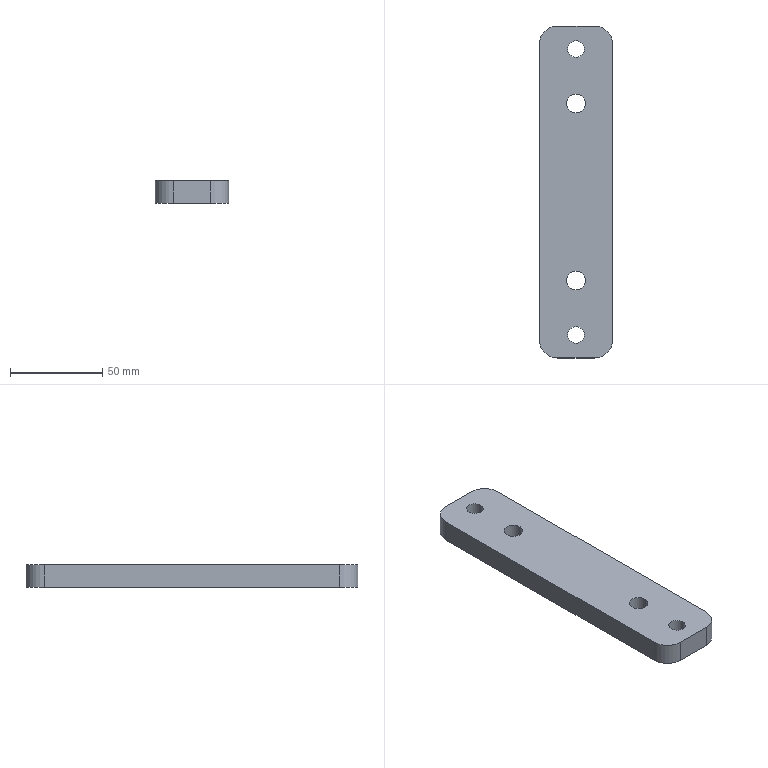Part | STEP file | Base plate 2_Default<Machined> | 1 solid | 18 faces | box 40 x 180 x 12 mm | volume 81882 mm3 | cylinder 12 | plane 6 | commonest cylinder face diameters 9 x4 10.2 x4 20 x4
STEP:
#1=CARTESIAN_POINT('',(-4.5,77.5,0.));
#2=VERTEX_POINT('',#1);
#3=CARTESIAN_POINT('',(4.5,77.5,0.));
#4=VERTEX_POINT('',#3);
#5=CARTESIAN_POINT('',(0.,77.5,0.));
#6=DIRECTION('',(0.,0.,1.));
#7=DIRECTION('',(1.,0.,0.));
#8=AXIS2_PLACEMENT_3D('',#5,#6,#7);
#9=CIRCLE('',#8,4.5);
#10=EDGE_CURVE('',#2,#4,#9,.T.);
#11=ORIENTED_EDGE('',*,*,#10,.F.);
#12=CARTESIAN_POINT('',(-4.5,77.5,12.));
#13=VERTEX_POINT('',#12);
#14=CARTESIAN_POINT('',(-4.5,77.5,12.));
#15=DIRECTION('',(0.,0.,1.));
#16=VECTOR('',#15,1000.);
#17=LINE('',#14,#16);
#18=EDGE_CURVE('',#2,#13,#17,.T.);
#19=ORIENTED_EDGE('',*,*,#18,.T.);
#20=CARTESIAN_POINT('',(4.5,77.5,12.));
#21=VERTEX_POINT('',#20);
#22=CARTESIAN_POINT('',(0.,77.5,12.));
#23=DIRECTION('',(0.,0.,1.));
#24=DIRECTION('',(1.,0.,0.));
#25=AXIS2_PLACEMENT_3D('',#22,#23,#24);
#26=CIRCLE('',#25,4.5);
#27=EDGE_CURVE('',#13,#21,#26,.T.);
#28=ORIENTED_EDGE('',*,*,#27,.T.);
#29=CARTESIAN_POINT('',(4.5,77.5,12.));
#30=DIRECTION('',(0.,0.,1.));
#31=VECTOR('',#30,1000.);
#32=LINE('',#29,#31);
#33=EDGE_CURVE('',#4,#21,#32,.T.);
#34=ORIENTED_EDGE('',*,*,#33,.F.);
#35=EDGE_LOOP('',(#11,#19,#28,#34));
#36=FACE_OUTER_BOUND('',#35,.T.);
#37=CARTESIAN_POINT('',(0.,77.5,12.));
#38=DIRECTION('',(0.,0.,1.));
#39=DIRECTION('',(1.,0.,0.));
#40=AXIS2_PLACEMENT_3D('',#37,#38,#39);
#41=CYLINDRICAL_SURFACE('',#40,4.5);
#42=ADVANCED_FACE('',(#36),#41,.F.);
#43=CARTESIAN_POINT('',(-4.5,-77.5,0.));
#44=VERTEX_POINT('',#43);
#45=CARTESIAN_POINT('',(4.5,-77.5,0.));
#46=VERTEX_POINT('',#45);
#47=CARTESIAN_POINT('',(0.,-77.5,0.));
#48=DIRECTION('',(0.,0.,1.));
#49=DIRECTION('',(1.,0.,0.));
#50=AXIS2_PLACEMENT_3D('',#47,#48,#49);
#51=CIRCLE('',#50,4.5);
#52=EDGE_CURVE('',#44,#46,#51,.T.);
#53=ORIENTED_EDGE('',*,*,#52,.F.);
#54=CARTESIAN_POINT('',(-4.5,-77.5,12.));
#55=VERTEX_POINT('',#54);
#56=CARTESIAN_POINT('',(-4.5,-77.5,12.));
#57=DIRECTION('',(0.,0.,1.));
#58=VECTOR('',#57,1000.);
#59=LINE('',#56,#58);
#60=EDGE_CURVE('',#44,#55,#59,.T.);
#61=ORIENTED_EDGE('',*,*,#60,.T.);
#62=CARTESIAN_POINT('',(4.5,-77.5,12.));
#63=VERTEX_POINT('',#62);
#64=CARTESIAN_POINT('',(0.,-77.5,12.));
#65=DIRECTION('',(0.,0.,1.));
#66=DIRECTION('',(1.,0.,0.));
#67=AXIS2_PLACEMENT_3D('',#64,#65,#66);
#68=CIRCLE('',#67,4.5);
#69=EDGE_CURVE('',#55,#63,#68,.T.);
#70=ORIENTED_EDGE('',*,*,#69,.T.);
#71=CARTESIAN_POINT('',(4.5,-77.5,12.));
#72=DIRECTION('',(0.,0.,1.));
#73=VECTOR('',#72,1000.);
#74=LINE('',#71,#73);
#75=EDGE_CURVE('',#46,#63,#74,.T.);
#76=ORIENTED_EDGE('',*,*,#75,.F.);
#77=EDGE_LOOP('',(#53,#61,#70,#76));
#78=FACE_OUTER_BOUND('',#77,.T.);
#79=CARTESIAN_POINT('',(0.,-77.5,12.));
#80=DIRECTION('',(0.,0.,1.));
#81=DIRECTION('',(1.,0.,0.));
#82=AXIS2_PLACEMENT_3D('',#79,#80,#81);
#83=CYLINDRICAL_SURFACE('',#82,4.5);
#84=ADVANCED_FACE('',(#78),#83,.F.);
#85=CARTESIAN_POINT('',(-5.1,48.,0.));
#86=VERTEX_POINT('',#85);
#87=CARTESIAN_POINT('',(5.1,48.,0.));
#88=VERTEX_POINT('',#87);
#89=CARTESIAN_POINT('',(0.,48.,0.));
#90=DIRECTION('',(0.,0.,1.));
#91=DIRECTION('',(1.,0.,0.));
#92=AXIS2_PLACEMENT_3D('',#89,#90,#91);
#93=CIRCLE('',#92,5.1);
#94=EDGE_CURVE('',#86,#88,#93,.T.);
#95=ORIENTED_EDGE('',*,*,#94,.F.);
#96=CARTESIAN_POINT('',(-5.1,48.,12.));
#97=VERTEX_POINT('',#96);
#98=CARTESIAN_POINT('',(-5.1,48.,12.));
#99=DIRECTION('',(0.,0.,1.));
#100=VECTOR('',#99,1000.);
#101=LINE('',#98,#100);
#102=EDGE_CURVE('',#86,#97,#101,.T.);
#103=ORIENTED_EDGE('',*,*,#102,.T.);
#104=CARTESIAN_POINT('',(5.1,48.,12.));
#105=VERTEX_POINT('',#104);
#106=CARTESIAN_POINT('',(0.,48.,12.));
#107=DIRECTION('',(0.,0.,1.));
#108=DIRECTION('',(1.,0.,0.));
#109=AXIS2_PLACEMENT_3D('',#106,#107,#108);
#110=CIRCLE('',#109,5.1);
#111=EDGE_CURVE('',#97,#105,#110,.T.);
#112=ORIENTED_EDGE('',*,*,#111,.T.);
#113=CARTESIAN_POINT('',(5.1,48.,12.));
#114=DIRECTION('',(0.,0.,1.));
#115=VECTOR('',#114,1000.);
#116=LINE('',#113,#115);
#117=EDGE_CURVE('',#88,#105,#116,.T.);
#118=ORIENTED_EDGE('',*,*,#117,.F.);
#119=EDGE_LOOP('',(#95,#103,#112,#118));
#120=FACE_OUTER_BOUND('',#119,.T.);
#121=CARTESIAN_POINT('',(0.,48.,12.));
#122=DIRECTION('',(0.,0.,1.));
#123=DIRECTION('',(1.,0.,0.));
#124=AXIS2_PLACEMENT_3D('',#121,#122,#123);
#125=CYLINDRICAL_SURFACE('',#124,5.1);
#126=ADVANCED_FACE('',(#120),#125,.F.);
#127=CARTESIAN_POINT('',(-5.1,-48.,0.));
#128=VERTEX_POINT('',#127);
#129=CARTESIAN_POINT('',(5.1,-48.,0.));
#130=VERTEX_POINT('',#129);
#131=CARTESIAN_POINT('',(0.,-48.,0.));
#132=DIRECTION('',(0.,0.,1.));
#133=DIRECTION('',(1.,0.,0.));
#134=AXIS2_PLACEMENT_3D('',#131,#132,#133);
#135=CIRCLE('',#134,5.1);
#136=EDGE_CURVE('',#128,#130,#135,.T.);
#137=ORIENTED_EDGE('',*,*,#136,.F.);
#138=CARTESIAN_POINT('',(-5.1,-48.,12.));
#139=VERTEX_POINT('',#138);
#140=CARTESIAN_POINT('',(-5.1,-48.,12.));
#141=DIRECTION('',(0.,0.,1.));
#142=VECTOR('',#141,1000.);
#143=LINE('',#140,#142);
#144=EDGE_CURVE('',#128,#139,#143,.T.);
#145=ORIENTED_EDGE('',*,*,#144,.T.);
#146=CARTESIAN_POINT('',(5.1,-48.,12.));
#147=VERTEX_POINT('',#146);
#148=CARTESIAN_POINT('',(0.,-48.,12.));
#149=DIRECTION('',(0.,0.,1.));
#150=DIRECTION('',(1.,0.,0.));
#151=AXIS2_PLACEMENT_3D('',#148,#149,#150);
#152=CIRCLE('',#151,5.1);
#153=EDGE_CURVE('',#139,#147,#152,.T.);
#154=ORIENTED_EDGE('',*,*,#153,.T.);
#155=CARTESIAN_POINT('',(5.1,-48.,12.));
#156=DIRECTION('',(0.,0.,1.));
#157=VECTOR('',#156,1000.);
#158=LINE('',#155,#157);
#159=EDGE_CURVE('',#130,#147,#158,.T.);
#160=ORIENTED_EDGE('',*,*,#159,.F.);
#161=EDGE_LOOP('',(#137,#145,#154,#160));
#162=FACE_OUTER_BOUND('',#161,.T.);
#163=CARTESIAN_POINT('',(0.,-48.,12.));
#164=DIRECTION('',(0.,0.,1.));
#165=DIRECTION('',(1.,0.,0.));
#166=AXIS2_PLACEMENT_3D('',#163,#164,#165);
#167=CYLINDRICAL_SURFACE('',#166,5.1);
#168=ADVANCED_FACE('',(#162),#167,.F.);
#169=CARTESIAN_POINT('',(20.,-80.,12.));
#170=VERTEX_POINT('',#169);
#171=CARTESIAN_POINT('',(20.,80.,12.));
#172=VERTEX_POINT('',#171);
#173=CARTESIAN_POINT('',(20.,90.,12.));
#174=DIRECTION('',(0.,1.,0.));
#175=VECTOR('',#174,1000.);
#176=LINE('',#173,#175);
#177=EDGE_CURVE('',#170,#172,#176,.T.);
#178=ORIENTED_EDGE('',*,*,#177,.F.);
#179=CARTESIAN_POINT('',(20.,-80.,0.));
#180=VERTEX_POINT('',#179);
#181=CARTESIAN_POINT('',(20.,-80.,12.));
#182=DIRECTION('',(0.,0.,-1.));
#183=VECTOR('',#182,1000.);
#184=LINE('',#181,#183);
#185=EDGE_CURVE('',#170,#180,#184,.T.);
#186=ORIENTED_EDGE('',*,*,#185,.T.);
#187=CARTESIAN_POINT('',(20.,80.,0.));
#188=VERTEX_POINT('',#187);
#189=CARTESIAN_POINT('',(20.,90.,0.));
#190=DIRECTION('',(0.,1.,0.));
#191=VECTOR('',#190,1000.);
#192=LINE('',#189,#191);
#193=EDGE_CURVE('',#180,#188,#192,.T.);
#194=ORIENTED_EDGE('',*,*,#193,.T.);
#195=CARTESIAN_POINT('',(20.,80.,12.));
#196=DIRECTION('',(0.,0.,1.));
#197=VECTOR('',#196,1000.);
#198=LINE('',#195,#197);
#199=EDGE_CURVE('',#188,#172,#198,.T.);
#200=ORIENTED_EDGE('',*,*,#199,.T.);
#201=EDGE_LOOP('',(#178,#186,#194,#200));
#202=FACE_OUTER_BOUND('',#201,.T.);
#203=CARTESIAN_POINT('',(20.,90.,12.));
#204=DIRECTION('',(-1.,0.,0.));
#205=DIRECTION('',(0.,-1.,0.));
#206=AXIS2_PLACEMENT_3D('',#203,#204,#205);
#207=PLANE('',#206);
#208=ADVANCED_FACE('',(#202),#207,.F.);
#209=CARTESIAN_POINT('',(10.,90.,12.));
#210=VERTEX_POINT('',#209);
#211=CARTESIAN_POINT('',(-10.,90.,12.));
#212=VERTEX_POINT('',#211);
#213=CARTESIAN_POINT('',(-20.,90.,12.));
#214=DIRECTION('',(-1.,0.,0.));
#215=VECTOR('',#214,1000.);
#216=LINE('',#213,#215);
#217=EDGE_CURVE('',#210,#212,#216,.T.);
#218=ORIENTED_EDGE('',*,*,#217,.F.);
#219=CARTESIAN_POINT('',(10.,90.,0.));
#220=VERTEX_POINT('',#219);
#221=CARTESIAN_POINT('',(10.,90.,12.));
#222=DIRECTION('',(0.,0.,-1.));
#223=VECTOR('',#222,1000.);
#224=LINE('',#221,#223);
#225=EDGE_CURVE('',#210,#220,#224,.T.);
#226=ORIENTED_EDGE('',*,*,#225,.T.);
#227=CARTESIAN_POINT('',(-10.,90.,0.));
#228=VERTEX_POINT('',#227);
#229=CARTESIAN_POINT('',(-20.,90.,0.));
#230=DIRECTION('',(-1.,0.,0.));
#231=VECTOR('',#230,1000.);
#232=LINE('',#229,#231);
#233=EDGE_CURVE('',#220,#228,#232,.T.);
#234=ORIENTED_EDGE('',*,*,#233,.T.);
#235=CARTESIAN_POINT('',(-10.,90.,12.));
#236=DIRECTION('',(0.,0.,1.));
#237=VECTOR('',#236,1000.);
#238=LINE('',#235,#237);
#239=EDGE_CURVE('',#228,#212,#238,.T.);
#240=ORIENTED_EDGE('',*,*,#239,.T.);
#241=EDGE_LOOP('',(#218,#226,#234,#240));
#242=FACE_OUTER_BOUND('',#241,.T.);
#243=CARTESIAN_POINT('',(-20.,90.,12.));
#244=DIRECTION('',(0.,-1.,0.));
#245=DIRECTION('',(0.,0.,-1.));
#246=AXIS2_PLACEMENT_3D('',#243,#244,#245);
#247=PLANE('',#246);
#248=ADVANCED_FACE('',(#242),#247,.F.);
#249=CARTESIAN_POINT('',(-20.,80.,0.));
#250=VERTEX_POINT('',#249);
#251=CARTESIAN_POINT('',(-20.,-80.,0.));
#252=VERTEX_POINT('',#251);
#253=CARTESIAN_POINT('',(-20.,90.,0.));
#254=DIRECTION('',(0.,-1.,0.));
#255=VECTOR('',#254,1000.);
#256=LINE('',#253,#255);
#257=EDGE_CURVE('',#250,#252,#256,.T.);
#258=ORIENTED_EDGE('',*,*,#257,.T.);
#259=CARTESIAN_POINT('',(-20.,-80.,12.));
#260=VERTEX_POINT('',#259);
#261=CARTESIAN_POINT('',(-20.,-80.,12.));
#262=DIRECTION('',(0.,0.,1.));
#263=VECTOR('',#262,1000.);
#264=LINE('',#261,#263);
#265=EDGE_CURVE('',#252,#260,#264,.T.);
#266=ORIENTED_EDGE('',*,*,#265,.T.);
#267=CARTESIAN_POINT('',(-20.,80.,12.));
#268=VERTEX_POINT('',#267);
#269=CARTESIAN_POINT('',(-20.,90.,12.));
#270=DIRECTION('',(0.,-1.,0.));
#271=VECTOR('',#270,1000.);
#272=LINE('',#269,#271);
#273=EDGE_CURVE('',#268,#260,#272,.T.);
#274=ORIENTED_EDGE('',*,*,#273,.F.);
#275=CARTESIAN_POINT('',(-20.,80.,12.));
#276=DIRECTION('',(0.,0.,-1.));
#277=VECTOR('',#276,1000.);
#278=LINE('',#275,#277);
#279=EDGE_CURVE('',#268,#250,#278,.T.);
#280=ORIENTED_EDGE('',*,*,#279,.T.);
#281=EDGE_LOOP('',(#258,#266,#274,#280));
#282=FACE_OUTER_BOUND('',#281,.T.);
#283=CARTESIAN_POINT('',(-20.,90.,12.));
#284=DIRECTION('',(1.,0.,0.));
#285=DIRECTION('',(0.,1.,0.));
#286=AXIS2_PLACEMENT_3D('',#283,#284,#285);
#287=PLANE('',#286);
#288=ADVANCED_FACE('',(#282),#287,.F.);
#289=CARTESIAN_POINT('',(-10.,-90.,0.));
#290=VERTEX_POINT('',#289);
#291=CARTESIAN_POINT('',(10.,-90.,0.));
#292=VERTEX_POINT('',#291);
#293=CARTESIAN_POINT('',(-20.,-90.,0.));
#294=DIRECTION('',(1.,0.,0.));
#295=VECTOR('',#294,1000.);
#296=LINE('',#293,#295);
#297=EDGE_CURVE('',#290,#292,#296,.T.);
#298=ORIENTED_EDGE('',*,*,#297,.T.);
#299=CARTESIAN_POINT('',(10.,-90.,12.));
#300=VERTEX_POINT('',#299);
#301=CARTESIAN_POINT('',(10.,-90.,12.));
#302=DIRECTION('',(0.,0.,1.));
#303=VECTOR('',#302,1000.);
#304=LINE('',#301,#303);
#305=EDGE_CURVE('',#292,#300,#304,.T.);
#306=ORIENTED_EDGE('',*,*,#305,.T.);
#307=CARTESIAN_POINT('',(-10.,-90.,12.));
#308=VERTEX_POINT('',#307);
#309=CARTESIAN_POINT('',(-20.,-90.,12.));
#310=DIRECTION('',(1.,0.,0.));
#311=VECTOR('',#310,1000.);
#312=LINE('',#309,#311);
#313=EDGE_CURVE('',#308,#300,#312,.T.);
#314=ORIENTED_EDGE('',*,*,#313,.F.);
#315=CARTESIAN_POINT('',(-10.,-90.,12.));
#316=DIRECTION('',(0.,0.,-1.));
#317=VECTOR('',#316,1000.);
#318=LINE('',#315,#317);
#319=EDGE_CURVE('',#308,#290,#318,.T.);
#320=ORIENTED_EDGE('',*,*,#319,.T.);
#321=EDGE_LOOP('',(#298,#306,#314,#320));
#322=FACE_OUTER_BOUND('',#321,.T.);
#323=CARTESIAN_POINT('',(-20.,-90.,12.));
#324=DIRECTION('',(0.,1.,0.));
#325=DIRECTION('',(0.,0.,1.));
#326=AXIS2_PLACEMENT_3D('',#323,#324,#325);
#327=PLANE('',#326);
#328=ADVANCED_FACE('',(#322),#327,.F.);
#329=CARTESIAN_POINT('',(0.,77.5,12.));
#330=DIRECTION('',(0.,0.,1.));
#331=DIRECTION('',(1.,0.,0.));
#332=AXIS2_PLACEMENT_3D('',#329,#330,#331);
#333=CIRCLE('',#332,4.5);
#334=EDGE_CURVE('',#21,#13,#333,.T.);
#335=ORIENTED_EDGE('',*,*,#334,.F.);
#336=ORIENTED_EDGE('',*,*,#27,.F.);
#337=EDGE_LOOP('',(#335,#336));
#338=FACE_BOUND('',#337,.T.);
#339=CARTESIAN_POINT('',(0.,-77.5,12.));
#340=DIRECTION('',(0.,0.,1.));
#341=DIRECTION('',(1.,0.,0.));
#342=AXIS2_PLACEMENT_3D('',#339,#340,#341);
#343=CIRCLE('',#342,4.5);
#344=EDGE_CURVE('',#63,#55,#343,.T.);
#345=ORIENTED_EDGE('',*,*,#344,.F.);
#346=ORIENTED_EDGE('',*,*,#69,.F.);
#347=EDGE_LOOP('',(#345,#346));
#348=FACE_BOUND('',#347,.T.);
#349=CARTESIAN_POINT('',(0.,48.,12.));
#350=DIRECTION('',(0.,0.,1.));
#351=DIRECTION('',(1.,0.,0.));
#352=AXIS2_PLACEMENT_3D('',#349,#350,#351);
#353=CIRCLE('',#352,5.1);
#354=EDGE_CURVE('',#105,#97,#353,.T.);
#355=ORIENTED_EDGE('',*,*,#354,.F.);
#356=ORIENTED_EDGE('',*,*,#111,.F.);
#357=EDGE_LOOP('',(#355,#356));
#358=FACE_BOUND('',#357,.T.);
#359=CARTESIAN_POINT('',(0.,-48.,12.));
#360=DIRECTION('',(0.,0.,1.));
#361=DIRECTION('',(1.,0.,0.));
#362=AXIS2_PLACEMENT_3D('',#359,#360,#361);
#363=CIRCLE('',#362,5.1);
#364=EDGE_CURVE('',#147,#139,#363,.T.);
#365=ORIENTED_EDGE('',*,*,#364,.F.);
#366=ORIENTED_EDGE('',*,*,#153,.F.);
#367=EDGE_LOOP('',(#365,#366));
#368=FACE_BOUND('',#367,.T.);
#369=ORIENTED_EDGE('',*,*,#313,.T.);
#370=CARTESIAN_POINT('',(10.,-80.,12.));
#371=DIRECTION('',(0.,0.,1.));
#372=DIRECTION('',(1.,0.,0.));
#373=AXIS2_PLACEMENT_3D('',#370,#371,#372);
#374=CIRCLE('',#373,10.);
#375=EDGE_CURVE('',#300,#170,#374,.T.);
#376=ORIENTED_EDGE('',*,*,#375,.T.);
#377=ORIENTED_EDGE('',*,*,#177,.T.);
#378=CARTESIAN_POINT('',(10.,80.,12.));
#379=DIRECTION('',(0.,0.,1.));
#380=DIRECTION('',(1.,0.,0.));
#381=AXIS2_PLACEMENT_3D('',#378,#379,#380);
#382=CIRCLE('',#381,10.);
#383=EDGE_CURVE('',#172,#210,#382,.T.);
#384=ORIENTED_EDGE('',*,*,#383,.T.);
#385=ORIENTED_EDGE('',*,*,#217,.T.);
#386=CARTESIAN_POINT('',(-10.,80.,12.));
#387=DIRECTION('',(0.,0.,1.));
#388=DIRECTION('',(1.,0.,0.));
#389=AXIS2_PLACEMENT_3D('',#386,#387,#388);
#390=CIRCLE('',#389,10.);
#391=EDGE_CURVE('',#212,#268,#390,.T.);
#392=ORIENTED_EDGE('',*,*,#391,.T.);
#393=ORIENTED_EDGE('',*,*,#273,.T.);
#394=CARTESIAN_POINT('',(-10.,-80.,12.));
#395=DIRECTION('',(0.,0.,1.));
#396=DIRECTION('',(1.,0.,0.));
#397=AXIS2_PLACEMENT_3D('',#394,#395,#396);
#398=CIRCLE('',#397,10.);
#399=EDGE_CURVE('',#260,#308,#398,.T.);
#400=ORIENTED_EDGE('',*,*,#399,.T.);
#401=EDGE_LOOP('',(#369,#376,#377,#384,#385,#392,#393,#400));
#402=FACE_OUTER_BOUND('',#401,.T.);
#403=CARTESIAN_POINT('',(0.,0.,12.));
#404=DIRECTION('',(0.,0.,1.));
#405=DIRECTION('',(1.,0.,0.));
#406=AXIS2_PLACEMENT_3D('',#403,#404,#405);
#407=PLANE('',#406);
#408=ADVANCED_FACE('',(#338,#348,#358,#368,#402),#407,.T.);
#409=CARTESIAN_POINT('',(0.,77.5,0.));
#410=DIRECTION('',(0.,0.,1.));
#411=DIRECTION('',(1.,0.,0.));
#412=AXIS2_PLACEMENT_3D('',#409,#410,#411);
#413=CIRCLE('',#412,4.5);
#414=EDGE_CURVE('',#4,#2,#413,.T.);
#415=ORIENTED_EDGE('',*,*,#414,.T.);
#416=ORIENTED_EDGE('',*,*,#10,.T.);
#417=EDGE_LOOP('',(#415,#416));
#418=FACE_BOUND('',#417,.T.);
#419=CARTESIAN_POINT('',(0.,-77.5,0.));
#420=DIRECTION('',(0.,0.,1.));
#421=DIRECTION('',(1.,0.,0.));
#422=AXIS2_PLACEMENT_3D('',#419,#420,#421);
#423=CIRCLE('',#422,4.5);
#424=EDGE_CURVE('',#46,#44,#423,.T.);
#425=ORIENTED_EDGE('',*,*,#424,.T.);
#426=ORIENTED_EDGE('',*,*,#52,.T.);
#427=EDGE_LOOP('',(#425,#426));
#428=FACE_BOUND('',#427,.T.);
#429=CARTESIAN_POINT('',(0.,48.,0.));
#430=DIRECTION('',(0.,0.,1.));
#431=DIRECTION('',(1.,0.,0.));
#432=AXIS2_PLACEMENT_3D('',#429,#430,#431);
#433=CIRCLE('',#432,5.1);
#434=EDGE_CURVE('',#88,#86,#433,.T.);
#435=ORIENTED_EDGE('',*,*,#434,.T.);
#436=ORIENTED_EDGE('',*,*,#94,.T.);
#437=EDGE_LOOP('',(#435,#436));
#438=FACE_BOUND('',#437,.T.);
#439=CARTESIAN_POINT('',(0.,-48.,0.));
#440=DIRECTION('',(0.,0.,1.));
#441=DIRECTION('',(1.,0.,0.));
#442=AXIS2_PLACEMENT_3D('',#439,#440,#441);
#443=CIRCLE('',#442,5.1);
#444=EDGE_CURVE('',#130,#128,#443,.T.);
#445=ORIENTED_EDGE('',*,*,#444,.T.);
#446=ORIENTED_EDGE('',*,*,#136,.T.);
#447=EDGE_LOOP('',(#445,#446));
#448=FACE_BOUND('',#447,.T.);
#449=ORIENTED_EDGE('',*,*,#193,.F.);
#450=CARTESIAN_POINT('',(10.,-80.,0.));
#451=DIRECTION('',(0.,0.,-1.));
#452=DIRECTION('',(1.,0.,0.));
#453=AXIS2_PLACEMENT_3D('',#450,#451,#452);
#454=CIRCLE('',#453,10.);
#455=EDGE_CURVE('',#180,#292,#454,.T.);
#456=ORIENTED_EDGE('',*,*,#455,.T.);
#457=ORIENTED_EDGE('',*,*,#297,.F.);
#458=CARTESIAN_POINT('',(-10.,-80.,0.));
#459=DIRECTION('',(0.,0.,-1.));
#460=DIRECTION('',(1.,0.,0.));
#461=AXIS2_PLACEMENT_3D('',#458,#459,#460);
#462=CIRCLE('',#461,10.);
#463=EDGE_CURVE('',#290,#252,#462,.T.);
#464=ORIENTED_EDGE('',*,*,#463,.T.);
#465=ORIENTED_EDGE('',*,*,#257,.F.);
#466=CARTESIAN_POINT('',(-10.,80.,0.));
#467=DIRECTION('',(0.,0.,-1.));
#468=DIRECTION('',(1.,0.,0.));
#469=AXIS2_PLACEMENT_3D('',#466,#467,#468);
#470=CIRCLE('',#469,10.);
#471=EDGE_CURVE('',#250,#228,#470,.T.);
#472=ORIENTED_EDGE('',*,*,#471,.T.);
#473=ORIENTED_EDGE('',*,*,#233,.F.);
#474=CARTESIAN_POINT('',(10.,80.,0.));
#475=DIRECTION('',(0.,0.,-1.));
#476=DIRECTION('',(1.,0.,0.));
#477=AXIS2_PLACEMENT_3D('',#474,#475,#476);
#478=CIRCLE('',#477,10.);
#479=EDGE_CURVE('',#220,#188,#478,.T.);
#480=ORIENTED_EDGE('',*,*,#479,.T.);
#481=EDGE_LOOP('',(#449,#456,#457,#464,#465,#472,#473,#480));
#482=FACE_OUTER_BOUND('',#481,.T.);
#483=CARTESIAN_POINT('',(0.,0.,0.));
#484=DIRECTION('',(0.,0.,1.));
#485=DIRECTION('',(1.,0.,0.));
#486=AXIS2_PLACEMENT_3D('',#483,#484,#485);
#487=PLANE('',#486);
#488=ADVANCED_FACE('',(#418,#428,#438,#448,#482),#487,.F.);
#489=ORIENTED_EDGE('',*,*,#144,.F.);
#490=ORIENTED_EDGE('',*,*,#444,.F.);
#491=ORIENTED_EDGE('',*,*,#159,.T.);
#492=ORIENTED_EDGE('',*,*,#364,.T.);
#493=EDGE_LOOP('',(#489,#490,#491,#492));
#494=FACE_OUTER_BOUND('',#493,.T.);
#495=CARTESIAN_POINT('',(0.,-48.,12.));
#496=DIRECTION('',(0.,0.,1.));
#497=DIRECTION('',(1.,0.,0.));
#498=AXIS2_PLACEMENT_3D('',#495,#496,#497);
#499=CYLINDRICAL_SURFACE('',#498,5.1);
#500=ADVANCED_FACE('',(#494),#499,.F.);
#501=ORIENTED_EDGE('',*,*,#102,.F.);
#502=ORIENTED_EDGE('',*,*,#434,.F.);
#503=ORIENTED_EDGE('',*,*,#117,.T.);
#504=ORIENTED_EDGE('',*,*,#354,.T.);
#505=EDGE_LOOP('',(#501,#502,#503,#504));
#506=FACE_OUTER_BOUND('',#505,.T.);
#507=CARTESIAN_POINT('',(0.,48.,12.));
#508=DIRECTION('',(0.,0.,1.));
#509=DIRECTION('',(1.,0.,0.));
#510=AXIS2_PLACEMENT_3D('',#507,#508,#509);
#511=CYLINDRICAL_SURFACE('',#510,5.1);
#512=ADVANCED_FACE('',(#506),#511,.F.);
#513=ORIENTED_EDGE('',*,*,#375,.F.);
#514=ORIENTED_EDGE('',*,*,#305,.F.);
#515=ORIENTED_EDGE('',*,*,#455,.F.);
#516=ORIENTED_EDGE('',*,*,#185,.F.);
#517=EDGE_LOOP('',(#513,#514,#515,#516));
#518=FACE_OUTER_BOUND('',#517,.T.);
#519=CARTESIAN_POINT('',(10.,-80.,12.));
#520=DIRECTION('',(0.,0.,-1.));
#521=DIRECTION('',(-1.,0.,0.));
#522=AXIS2_PLACEMENT_3D('',#519,#520,#521);
#523=CYLINDRICAL_SURFACE('',#522,10.);
#524=ADVANCED_FACE('',(#518),#523,.T.);
#525=ORIENTED_EDGE('',*,*,#399,.F.);
#526=ORIENTED_EDGE('',*,*,#265,.F.);
#527=ORIENTED_EDGE('',*,*,#463,.F.);
#528=ORIENTED_EDGE('',*,*,#319,.F.);
#529=EDGE_LOOP('',(#525,#526,#527,#528));
#530=FACE_OUTER_BOUND('',#529,.T.);
#531=CARTESIAN_POINT('',(-10.,-80.,12.));
#532=DIRECTION('',(0.,0.,-1.));
#533=DIRECTION('',(-1.,0.,0.));
#534=AXIS2_PLACEMENT_3D('',#531,#532,#533);
#535=CYLINDRICAL_SURFACE('',#534,10.);
#536=ADVANCED_FACE('',(#530),#535,.T.);
#537=ORIENTED_EDGE('',*,*,#383,.F.);
#538=ORIENTED_EDGE('',*,*,#199,.F.);
#539=ORIENTED_EDGE('',*,*,#479,.F.);
#540=ORIENTED_EDGE('',*,*,#225,.F.);
#541=EDGE_LOOP('',(#537,#538,#539,#540));
#542=FACE_OUTER_BOUND('',#541,.T.);
#543=CARTESIAN_POINT('',(10.,80.,12.));
#544=DIRECTION('',(0.,0.,-1.));
#545=DIRECTION('',(-1.,0.,0.));
#546=AXIS2_PLACEMENT_3D('',#543,#544,#545);
#547=CYLINDRICAL_SURFACE('',#546,10.);
#548=ADVANCED_FACE('',(#542),#547,.T.);
#549=ORIENTED_EDGE('',*,*,#391,.F.);
#550=ORIENTED_EDGE('',*,*,#239,.F.);
#551=ORIENTED_EDGE('',*,*,#471,.F.);
#552=ORIENTED_EDGE('',*,*,#279,.F.);
#553=EDGE_LOOP('',(#549,#550,#551,#552));
#554=FACE_OUTER_BOUND('',#553,.T.);
#555=CARTESIAN_POINT('',(-10.,80.,12.));
#556=DIRECTION('',(0.,0.,-1.));
#557=DIRECTION('',(-1.,0.,0.));
#558=AXIS2_PLACEMENT_3D('',#555,#556,#557);
#559=CYLINDRICAL_SURFACE('',#558,10.);
#560=ADVANCED_FACE('',(#554),#559,.T.);
#561=ORIENTED_EDGE('',*,*,#60,.F.);
#562=ORIENTED_EDGE('',*,*,#424,.F.);
#563=ORIENTED_EDGE('',*,*,#75,.T.);
#564=ORIENTED_EDGE('',*,*,#344,.T.);
#565=EDGE_LOOP('',(#561,#562,#563,#564));
#566=FACE_OUTER_BOUND('',#565,.T.);
#567=CARTESIAN_POINT('',(0.,-77.5,12.));
#568=DIRECTION('',(0.,0.,1.));
#569=DIRECTION('',(1.,0.,0.));
#570=AXIS2_PLACEMENT_3D('',#567,#568,#569);
#571=CYLINDRICAL_SURFACE('',#570,4.5);
#572=ADVANCED_FACE('',(#566),#571,.F.);
#573=ORIENTED_EDGE('',*,*,#18,.F.);
#574=ORIENTED_EDGE('',*,*,#414,.F.);
#575=ORIENTED_EDGE('',*,*,#33,.T.);
#576=ORIENTED_EDGE('',*,*,#334,.T.);
#577=EDGE_LOOP('',(#573,#574,#575,#576));
#578=FACE_OUTER_BOUND('',#577,.T.);
#579=CARTESIAN_POINT('',(0.,77.5,12.));
#580=DIRECTION('',(0.,0.,1.));
#581=DIRECTION('',(1.,0.,0.));
#582=AXIS2_PLACEMENT_3D('',#579,#580,#581);
#583=CYLINDRICAL_SURFACE('',#582,4.5);
#584=ADVANCED_FACE('',(#578),#583,.F.);
#585=CLOSED_SHELL('',(#42,#84,#126,#168,#208,#248,#288,#328,#408,#488,#500,#512,#524,#536,#548,#560,#572,#584));
#586=MANIFOLD_SOLID_BREP('',#585);
#587=CARTESIAN_POINT('',(0.,0.,0.));
#588=DIRECTION('',(0.,0.,1.));
#589=DIRECTION('',(1.,0.,0.));
#590=AXIS2_PLACEMENT_3D('',#587,#588,#589);
#591=(LENGTH_UNIT()NAMED_UNIT(*)SI_UNIT(.MILLI.,.METRE.));
#592=UNCERTAINTY_MEASURE_WITH_UNIT(LENGTH_MEASURE(0.00001),#591,'','');
#593=(NAMED_UNIT(*)PLANE_ANGLE_UNIT()SI_UNIT($,.RADIAN.));
#594=(NAMED_UNIT(*)SI_UNIT($,.STERADIAN.)SOLID_ANGLE_UNIT());
#595=(GEOMETRIC_REPRESENTATION_CONTEXT(3)GLOBAL_UNCERTAINTY_ASSIGNED_CONTEXT((#592))GLOBAL_UNIT_ASSIGNED_CONTEXT((#591,#593,#594))REPRESENTATION_CONTEXT('',''));
#596=ADVANCED_BREP_SHAPE_REPRESENTATION('',(#586,#590),#595);